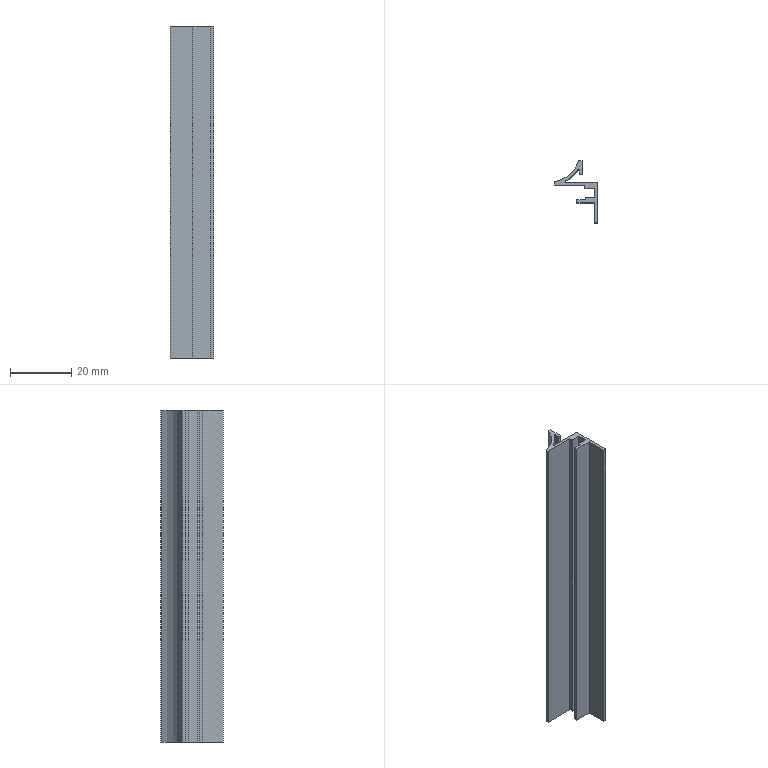Part | SolidWorks | features MoveFace 2, BaseBody 1, ICE 1 | 1 solid | 27 faces | box 14 x 20.3 x 108 mm | volume 5499 mm3 | plane 20 | cylinder 7 | commonest cylinder face diameters 0.387 x2 0.8 x2 0.4 x1 20 x1 22 x1
STEP:
#1=CARTESIAN_POINT('',(-5.304,-0.625,-205.));
#2=VERTEX_POINT('',#1);
#3=CARTESIAN_POINT('',(-5.449,-0.8125,-205.));
#4=VERTEX_POINT('',#3);
#5=CARTESIAN_POINT('',(-5.255,-0.8125,-205.));
#6=DIRECTION('',(0.,0.,1.));
#7=DIRECTION('',(-1.,0.,0.));
#8=AXIS2_PLACEMENT_3D('',#5,#6,#7);
#9=CIRCLE('',#8,0.1937);
#10=EDGE_CURVE('',#2,#4,#9,.T.);
#11=ORIENTED_EDGE('',*,*,#10,.T.);
#12=CARTESIAN_POINT('',(-5.449,-0.8125,-313.));
#13=VERTEX_POINT('',#12);
#14=CARTESIAN_POINT('',(-5.449,-0.8125,230.));
#15=DIRECTION('',(0.,0.,-1.));
#16=VECTOR('',#15,1000.);
#17=LINE('',#14,#16);
#18=EDGE_CURVE('',#4,#13,#17,.T.);
#19=ORIENTED_EDGE('',*,*,#18,.T.);
#20=CARTESIAN_POINT('',(-5.304,-0.625,-313.));
#21=VERTEX_POINT('',#20);
#22=CARTESIAN_POINT('',(-5.255,-0.8125,-313.));
#23=DIRECTION('',(0.,0.,-1.));
#24=DIRECTION('',(1.,0.,0.));
#25=AXIS2_PLACEMENT_3D('',#22,#23,#24);
#26=CIRCLE('',#25,0.1937);
#27=EDGE_CURVE('',#13,#21,#26,.T.);
#28=ORIENTED_EDGE('',*,*,#27,.T.);
#29=CARTESIAN_POINT('',(-5.304,-0.625,230.));
#30=DIRECTION('',(0.,0.,-1.));
#31=VECTOR('',#30,1000.);
#32=LINE('',#29,#31);
#33=EDGE_CURVE('',#2,#21,#32,.T.);
#34=ORIENTED_EDGE('',*,*,#33,.F.);
#35=EDGE_LOOP('',(#11,#19,#28,#34));
#36=FACE_OUTER_BOUND('',#35,.T.);
#37=CARTESIAN_POINT('',(-5.255,-0.8125,230.));
#38=DIRECTION('',(0.,0.,-1.));
#39=DIRECTION('',(-1.,0.,0.));
#40=AXIS2_PLACEMENT_3D('',#37,#38,#39);
#41=CYLINDRICAL_SURFACE('',#40,0.1937);
#42=ADVANCED_FACE('',(#36),#41,.F.);
#43=CARTESIAN_POINT('',(5.,-1.,-313.));
#44=VERTEX_POINT('',#43);
#45=CARTESIAN_POINT('',(5.,-14.3,-313.));
#46=VERTEX_POINT('',#45);
#47=CARTESIAN_POINT('',(5.,29.623,-313.));
#48=DIRECTION('',(0.,-1.,0.));
#49=VECTOR('',#48,1000.);
#50=LINE('',#47,#49);
#51=EDGE_CURVE('',#44,#46,#50,.T.);
#52=ORIENTED_EDGE('',*,*,#51,.F.);
#53=CARTESIAN_POINT('',(5.,-1.,-205.));
#54=VERTEX_POINT('',#53);
#55=CARTESIAN_POINT('',(5.,-1.,230.));
#56=DIRECTION('',(0.,0.,-1.));
#57=VECTOR('',#56,1000.);
#58=LINE('',#55,#57);
#59=EDGE_CURVE('',#54,#44,#58,.T.);
#60=ORIENTED_EDGE('',*,*,#59,.F.);
#61=CARTESIAN_POINT('',(5.,-14.3,-205.));
#62=VERTEX_POINT('',#61);
#63=CARTESIAN_POINT('',(5.,29.623,-205.));
#64=DIRECTION('',(0.,1.,0.));
#65=VECTOR('',#64,1000.);
#66=LINE('',#63,#65);
#67=EDGE_CURVE('',#62,#54,#66,.T.);
#68=ORIENTED_EDGE('',*,*,#67,.F.);
#69=CARTESIAN_POINT('',(5.,-14.3,230.));
#70=DIRECTION('',(0.,0.,1.));
#71=VECTOR('',#70,1000.);
#72=LINE('',#69,#71);
#73=EDGE_CURVE('',#46,#62,#72,.T.);
#74=ORIENTED_EDGE('',*,*,#73,.F.);
#75=EDGE_LOOP('',(#52,#60,#68,#74));
#76=FACE_OUTER_BOUND('',#75,.T.);
#77=CARTESIAN_POINT('',(5.,-14.3,230.));
#78=DIRECTION('',(-1.,0.,0.));
#79=DIRECTION('',(0.,0.,1.));
#80=AXIS2_PLACEMENT_3D('',#77,#78,#79);
#81=PLANE('',#80);
#82=ADVANCED_FACE('',(#76),#81,.F.);
#83=CARTESIAN_POINT('',(-9.,-2.,-313.));
#84=VERTEX_POINT('',#83);
#85=CARTESIAN_POINT('',(-9.,-2.,-205.));
#86=VERTEX_POINT('',#85);
#87=CARTESIAN_POINT('',(-9.,-2.,230.));
#88=DIRECTION('',(0.,0.,1.));
#89=VECTOR('',#88,1000.);
#90=LINE('',#87,#89);
#91=EDGE_CURVE('',#84,#86,#90,.T.);
#92=ORIENTED_EDGE('',*,*,#91,.F.);
#93=CARTESIAN_POINT('',(0.9,-2.,-313.));
#94=VERTEX_POINT('',#93);
#95=CARTESIAN_POINT('',(5.,-2.,-313.));
#96=DIRECTION('',(-1.,0.,0.));
#97=VECTOR('',#96,1000.);
#98=LINE('',#95,#97);
#99=EDGE_CURVE('',#94,#84,#98,.T.);
#100=ORIENTED_EDGE('',*,*,#99,.F.);
#101=CARTESIAN_POINT('',(0.9,-2.,-205.));
#102=VERTEX_POINT('',#101);
#103=CARTESIAN_POINT('',(0.9,-2.,230.));
#104=DIRECTION('',(0.,0.,-1.));
#105=VECTOR('',#104,1000.);
#106=LINE('',#103,#105);
#107=EDGE_CURVE('',#102,#94,#106,.T.);
#108=ORIENTED_EDGE('',*,*,#107,.F.);
#109=CARTESIAN_POINT('',(5.,-2.,-205.));
#110=DIRECTION('',(1.,0.,0.));
#111=VECTOR('',#110,1000.);
#112=LINE('',#109,#111);
#113=EDGE_CURVE('',#86,#102,#112,.T.);
#114=ORIENTED_EDGE('',*,*,#113,.F.);
#115=EDGE_LOOP('',(#92,#100,#108,#114));
#116=FACE_OUTER_BOUND('',#115,.T.);
#117=CARTESIAN_POINT('',(-9.,-2.,230.));
#118=DIRECTION('',(0.,1.,0.));
#119=DIRECTION('',(0.,0.,1.));
#120=AXIS2_PLACEMENT_3D('',#117,#118,#119);
#121=PLANE('',#120);
#122=ADVANCED_FACE('',(#116),#121,.F.);
#123=CARTESIAN_POINT('',(4.,-6.,-205.));
#124=VERTEX_POINT('',#123);
#125=CARTESIAN_POINT('',(4.,-3.,-205.));
#126=VERTEX_POINT('',#125);
#127=CARTESIAN_POINT('',(4.,-3.,-205.));
#128=DIRECTION('',(0.,1.,0.));
#129=VECTOR('',#128,1000.);
#130=LINE('',#127,#129);
#131=EDGE_CURVE('',#124,#126,#130,.T.);
#132=ORIENTED_EDGE('',*,*,#131,.F.);
#133=CARTESIAN_POINT('',(1.,-6.,-205.));
#134=VERTEX_POINT('',#133);
#135=CARTESIAN_POINT('',(4.,-6.,-205.));
#136=DIRECTION('',(1.,0.,0.));
#137=VECTOR('',#136,1000.);
#138=LINE('',#135,#137);
#139=EDGE_CURVE('',#134,#124,#138,.T.);
#140=ORIENTED_EDGE('',*,*,#139,.F.);
#141=CARTESIAN_POINT('',(1.,-6.7,-205.));
#142=VERTEX_POINT('',#141);
#143=CARTESIAN_POINT('',(1.,29.623,-205.));
#144=DIRECTION('',(0.,-1.,0.));
#145=VECTOR('',#144,1000.);
#146=LINE('',#143,#145);
#147=EDGE_CURVE('',#134,#142,#146,.T.);
#148=ORIENTED_EDGE('',*,*,#147,.T.);
#149=CARTESIAN_POINT('',(-1.7,-6.7,-205.));
#150=VERTEX_POINT('',#149);
#151=CARTESIAN_POINT('',(1.,-6.7,-205.));
#152=DIRECTION('',(1.,0.,0.));
#153=VECTOR('',#152,1000.);
#154=LINE('',#151,#153);
#155=EDGE_CURVE('',#150,#142,#154,.T.);
#156=ORIENTED_EDGE('',*,*,#155,.F.);
#157=CARTESIAN_POINT('',(-1.7,-7.7,-205.));
#158=VERTEX_POINT('',#157);
#159=CARTESIAN_POINT('',(-1.7,29.623,-205.));
#160=DIRECTION('',(0.,-1.,0.));
#161=VECTOR('',#160,1000.);
#162=LINE('',#159,#161);
#163=EDGE_CURVE('',#150,#158,#162,.T.);
#164=ORIENTED_EDGE('',*,*,#163,.T.);
#165=CARTESIAN_POINT('',(4.,-7.7,-205.));
#166=VERTEX_POINT('',#165);
#167=CARTESIAN_POINT('',(-1.7,-7.7,-205.));
#168=DIRECTION('',(-1.,0.,0.));
#169=VECTOR('',#168,1000.);
#170=LINE('',#167,#169);
#171=EDGE_CURVE('',#166,#158,#170,.T.);
#172=ORIENTED_EDGE('',*,*,#171,.F.);
#173=CARTESIAN_POINT('',(4.,-14.3,-205.));
#174=VERTEX_POINT('',#173);
#175=CARTESIAN_POINT('',(4.,-7.7,-205.));
#176=DIRECTION('',(0.,1.,0.));
#177=VECTOR('',#176,1000.);
#178=LINE('',#175,#177);
#179=EDGE_CURVE('',#174,#166,#178,.T.);
#180=ORIENTED_EDGE('',*,*,#179,.F.);
#181=CARTESIAN_POINT('',(4.,-14.3,-205.));
#182=DIRECTION('',(-1.,0.,0.));
#183=VECTOR('',#182,1000.);
#184=LINE('',#181,#183);
#185=EDGE_CURVE('',#62,#174,#184,.T.);
#186=ORIENTED_EDGE('',*,*,#185,.F.);
#187=ORIENTED_EDGE('',*,*,#67,.T.);
#188=CARTESIAN_POINT('',(-5.207,-1.,-205.));
#189=VERTEX_POINT('',#188);
#190=CARTESIAN_POINT('',(5.,-1.,-205.));
#191=DIRECTION('',(1.,0.,0.));
#192=VECTOR('',#191,1000.);
#193=LINE('',#190,#192);
#194=EDGE_CURVE('',#189,#54,#193,.T.);
#195=ORIENTED_EDGE('',*,*,#194,.F.);
#196=CARTESIAN_POINT('',(-5.255,-0.8125,-205.));
#197=DIRECTION('',(0.,0.,1.));
#198=DIRECTION('',(-1.,0.,0.));
#199=AXIS2_PLACEMENT_3D('',#196,#197,#198);
#200=CIRCLE('',#199,0.1937);
#201=EDGE_CURVE('',#4,#189,#200,.T.);
#202=ORIENTED_EDGE('',*,*,#201,.F.);
#203=ORIENTED_EDGE('',*,*,#10,.F.);
#204=CARTESIAN_POINT('',(-1.368,3.063,-205.));
#205=VERTEX_POINT('',#204);
#206=CARTESIAN_POINT('',(-10.628,9.,-205.));
#207=DIRECTION('',(0.,0.,1.));
#208=DIRECTION('',(-1.,0.,0.));
#209=AXIS2_PLACEMENT_3D('',#206,#207,#208);
#210=CIRCLE('',#209,11.);
#211=EDGE_CURVE('',#2,#205,#210,.T.);
#212=ORIENTED_EDGE('',*,*,#211,.T.);
#213=CARTESIAN_POINT('',(-1.,2.955,-205.));
#214=VERTEX_POINT('',#213);
#215=CARTESIAN_POINT('',(-1.2,2.955,-205.));
#216=DIRECTION('',(0.,0.,1.));
#217=DIRECTION('',(-1.,0.,0.));
#218=AXIS2_PLACEMENT_3D('',#215,#216,#217);
#219=CIRCLE('',#218,0.2);
#220=EDGE_CURVE('',#214,#205,#219,.T.);
#221=ORIENTED_EDGE('',*,*,#220,.F.);
#222=CARTESIAN_POINT('',(-1.,1.5,-205.));
#223=VERTEX_POINT('',#222);
#224=CARTESIAN_POINT('',(-1.,2.955,-205.));
#225=DIRECTION('',(0.,1.,0.));
#226=VECTOR('',#225,1000.);
#227=LINE('',#224,#226);
#228=EDGE_CURVE('',#223,#214,#227,.T.);
#229=ORIENTED_EDGE('',*,*,#228,.F.);
#230=CARTESIAN_POINT('',(0.,1.5,-205.));
#231=VERTEX_POINT('',#230);
#232=CARTESIAN_POINT('',(-1.,1.5,-205.));
#233=DIRECTION('',(-1.,0.,0.));
#234=VECTOR('',#233,1000.);
#235=LINE('',#232,#234);
#236=EDGE_CURVE('',#231,#223,#235,.T.);
#237=ORIENTED_EDGE('',*,*,#236,.F.);
#238=CARTESIAN_POINT('',(0.,6.,-205.));
#239=VERTEX_POINT('',#238);
#240=CARTESIAN_POINT('',(0.,1.5,-205.));
#241=DIRECTION('',(0.,-1.,0.));
#242=VECTOR('',#241,1000.);
#243=LINE('',#240,#242);
#244=EDGE_CURVE('',#239,#231,#243,.T.);
#245=ORIENTED_EDGE('',*,*,#244,.F.);
#246=CARTESIAN_POINT('',(-0.8,6.,-205.));
#247=VERTEX_POINT('',#246);
#248=CARTESIAN_POINT('',(0.,6.,-205.));
#249=DIRECTION('',(1.,0.,0.));
#250=VECTOR('',#249,1000.);
#251=LINE('',#248,#250);
#252=EDGE_CURVE('',#247,#239,#251,.T.);
#253=ORIENTED_EDGE('',*,*,#252,.F.);
#254=CARTESIAN_POINT('',(-1.178,5.731,-205.));
#255=VERTEX_POINT('',#254);
#256=CARTESIAN_POINT('',(-0.8,5.6,-205.));
#257=DIRECTION('',(0.,0.,1.));
#258=DIRECTION('',(-1.,0.,0.));
#259=AXIS2_PLACEMENT_3D('',#256,#257,#258);
#260=CIRCLE('',#259,0.4);
#261=EDGE_CURVE('',#247,#255,#260,.T.);
#262=ORIENTED_EDGE('',*,*,#261,.T.);
#263=CARTESIAN_POINT('',(-8.678,-0.8077,-205.));
#264=VERTEX_POINT('',#263);
#265=CARTESIAN_POINT('',(-10.628,9.,-205.));
#266=DIRECTION('',(0.,0.,1.));
#267=DIRECTION('',(-1.,0.,0.));
#268=AXIS2_PLACEMENT_3D('',#265,#266,#267);
#269=CIRCLE('',#268,10.);
#270=EDGE_CURVE('',#264,#255,#269,.T.);
#271=ORIENTED_EDGE('',*,*,#270,.F.);
#272=CARTESIAN_POINT('',(-9.,-1.2,-205.));
#273=VERTEX_POINT('',#272);
#274=CARTESIAN_POINT('',(-8.6,-1.2,-205.));
#275=DIRECTION('',(0.,0.,1.));
#276=DIRECTION('',(-1.,0.,0.));
#277=AXIS2_PLACEMENT_3D('',#274,#275,#276);
#278=CIRCLE('',#277,0.4);
#279=EDGE_CURVE('',#264,#273,#278,.T.);
#280=ORIENTED_EDGE('',*,*,#279,.T.);
#281=CARTESIAN_POINT('',(-9.,29.623,-205.));
#282=DIRECTION('',(0.,-1.,0.));
#283=VECTOR('',#282,1000.);
#284=LINE('',#281,#283);
#285=EDGE_CURVE('',#273,#86,#284,.T.);
#286=ORIENTED_EDGE('',*,*,#285,.T.);
#287=ORIENTED_EDGE('',*,*,#113,.T.);
#288=CARTESIAN_POINT('',(0.9,-3.,-205.));
#289=VERTEX_POINT('',#288);
#290=CARTESIAN_POINT('',(0.9,-2.,-205.));
#291=DIRECTION('',(0.,1.,0.));
#292=VECTOR('',#291,1000.);
#293=LINE('',#290,#292);
#294=EDGE_CURVE('',#289,#102,#293,.T.);
#295=ORIENTED_EDGE('',*,*,#294,.F.);
#296=CARTESIAN_POINT('',(0.9,-3.,-205.));
#297=DIRECTION('',(-1.,0.,0.));
#298=VECTOR('',#297,1000.);
#299=LINE('',#296,#298);
#300=EDGE_CURVE('',#126,#289,#299,.T.);
#301=ORIENTED_EDGE('',*,*,#300,.F.);
#302=EDGE_LOOP('',(#132,#140,#148,#156,#164,#172,#180,#186,#187,#195,#202,#203,#212,#221,#229,#237,#245,#253,#262,#271,#280,#286,#287,#295,#301));
#303=FACE_OUTER_BOUND('',#302,.T.);
#304=CARTESIAN_POINT('',(5.,29.623,-205.));
#305=DIRECTION('',(0.,0.,-1.));
#306=DIRECTION('',(-1.,0.,0.));
#307=AXIS2_PLACEMENT_3D('',#304,#305,#306);
#308=PLANE('',#307);
#309=ADVANCED_FACE('',(#303),#308,.F.);
#310=ORIENTED_EDGE('',*,*,#185,.T.);
#311=CARTESIAN_POINT('',(4.,-14.3,-313.));
#312=VERTEX_POINT('',#311);
#313=CARTESIAN_POINT('',(4.,-14.3,230.));
#314=DIRECTION('',(0.,0.,1.));
#315=VECTOR('',#314,1000.);
#316=LINE('',#313,#315);
#317=EDGE_CURVE('',#312,#174,#316,.T.);
#318=ORIENTED_EDGE('',*,*,#317,.F.);
#319=CARTESIAN_POINT('',(5.,-14.3,-313.));
#320=DIRECTION('',(-1.,0.,0.));
#321=VECTOR('',#320,1000.);
#322=LINE('',#319,#321);
#323=EDGE_CURVE('',#46,#312,#322,.T.);
#324=ORIENTED_EDGE('',*,*,#323,.F.);
#325=ORIENTED_EDGE('',*,*,#73,.T.);
#326=EDGE_LOOP('',(#310,#318,#324,#325));
#327=FACE_OUTER_BOUND('',#326,.T.);
#328=CARTESIAN_POINT('',(4.,-14.3,230.));
#329=DIRECTION('',(0.,1.,0.));
#330=DIRECTION('',(0.,0.,1.));
#331=AXIS2_PLACEMENT_3D('',#328,#329,#330);
#332=PLANE('',#331);
#333=ADVANCED_FACE('',(#327),#332,.F.);
#334=ORIENTED_EDGE('',*,*,#51,.T.);
#335=ORIENTED_EDGE('',*,*,#323,.T.);
#336=CARTESIAN_POINT('',(4.,-7.7,-313.));
#337=VERTEX_POINT('',#336);
#338=CARTESIAN_POINT('',(4.,-7.7,-313.));
#339=DIRECTION('',(0.,-1.,0.));
#340=VECTOR('',#339,1000.);
#341=LINE('',#338,#340);
#342=EDGE_CURVE('',#337,#312,#341,.T.);
#343=ORIENTED_EDGE('',*,*,#342,.F.);
#344=CARTESIAN_POINT('',(-1.7,-7.7,-313.));
#345=VERTEX_POINT('',#344);
#346=CARTESIAN_POINT('',(-1.7,-7.7,-313.));
#347=DIRECTION('',(1.,0.,0.));
#348=VECTOR('',#347,1000.);
#349=LINE('',#346,#348);
#350=EDGE_CURVE('',#345,#337,#349,.T.);
#351=ORIENTED_EDGE('',*,*,#350,.F.);
#352=CARTESIAN_POINT('',(-1.7,-6.7,-313.));
#353=VERTEX_POINT('',#352);
#354=CARTESIAN_POINT('',(-1.7,29.623,-313.));
#355=DIRECTION('',(0.,1.,0.));
#356=VECTOR('',#355,1000.);
#357=LINE('',#354,#356);
#358=EDGE_CURVE('',#345,#353,#357,.T.);
#359=ORIENTED_EDGE('',*,*,#358,.T.);
#360=CARTESIAN_POINT('',(1.,-6.7,-313.));
#361=VERTEX_POINT('',#360);
#362=CARTESIAN_POINT('',(1.,-6.7,-313.));
#363=DIRECTION('',(-1.,0.,0.));
#364=VECTOR('',#363,1000.);
#365=LINE('',#362,#364);
#366=EDGE_CURVE('',#361,#353,#365,.T.);
#367=ORIENTED_EDGE('',*,*,#366,.F.);
#368=CARTESIAN_POINT('',(1.,-6.,-313.));
#369=VERTEX_POINT('',#368);
#370=CARTESIAN_POINT('',(1.,29.623,-313.));
#371=DIRECTION('',(0.,1.,0.));
#372=VECTOR('',#371,1000.);
#373=LINE('',#370,#372);
#374=EDGE_CURVE('',#361,#369,#373,.T.);
#375=ORIENTED_EDGE('',*,*,#374,.T.);
#376=CARTESIAN_POINT('',(4.,-6.,-313.));
#377=VERTEX_POINT('',#376);
#378=CARTESIAN_POINT('',(4.,-6.,-313.));
#379=DIRECTION('',(-1.,0.,0.));
#380=VECTOR('',#379,1000.);
#381=LINE('',#378,#380);
#382=EDGE_CURVE('',#377,#369,#381,.T.);
#383=ORIENTED_EDGE('',*,*,#382,.F.);
#384=CARTESIAN_POINT('',(4.,-3.,-313.));
#385=VERTEX_POINT('',#384);
#386=CARTESIAN_POINT('',(4.,-3.,-313.));
#387=DIRECTION('',(0.,-1.,0.));
#388=VECTOR('',#387,1000.);
#389=LINE('',#386,#388);
#390=EDGE_CURVE('',#385,#377,#389,.T.);
#391=ORIENTED_EDGE('',*,*,#390,.F.);
#392=CARTESIAN_POINT('',(0.9,-3.,-313.));
#393=VERTEX_POINT('',#392);
#394=CARTESIAN_POINT('',(0.9,-3.,-313.));
#395=DIRECTION('',(1.,0.,0.));
#396=VECTOR('',#395,1000.);
#397=LINE('',#394,#396);
#398=EDGE_CURVE('',#393,#385,#397,.T.);
#399=ORIENTED_EDGE('',*,*,#398,.F.);
#400=CARTESIAN_POINT('',(0.9,-2.,-313.));
#401=DIRECTION('',(0.,-1.,0.));
#402=VECTOR('',#401,1000.);
#403=LINE('',#400,#402);
#404=EDGE_CURVE('',#94,#393,#403,.T.);
#405=ORIENTED_EDGE('',*,*,#404,.F.);
#406=ORIENTED_EDGE('',*,*,#99,.T.);
#407=CARTESIAN_POINT('',(-9.,-1.2,-313.));
#408=VERTEX_POINT('',#407);
#409=CARTESIAN_POINT('',(-9.,-1.2,-313.));
#410=DIRECTION('',(0.,-1.,0.));
#411=VECTOR('',#410,1000.);
#412=LINE('',#409,#411);
#413=EDGE_CURVE('',#408,#84,#412,.T.);
#414=ORIENTED_EDGE('',*,*,#413,.F.);
#415=CARTESIAN_POINT('',(-8.678,-0.8077,-313.));
#416=VERTEX_POINT('',#415);
#417=CARTESIAN_POINT('',(-8.6,-1.2,-313.));
#418=DIRECTION('',(0.,0.,-1.));
#419=DIRECTION('',(1.,0.,0.));
#420=AXIS2_PLACEMENT_3D('',#417,#418,#419);
#421=CIRCLE('',#420,0.4);
#422=EDGE_CURVE('',#408,#416,#421,.T.);
#423=ORIENTED_EDGE('',*,*,#422,.T.);
#424=CARTESIAN_POINT('',(-1.178,5.731,-313.));
#425=VERTEX_POINT('',#424);
#426=CARTESIAN_POINT('',(-10.628,9.,-313.));
#427=DIRECTION('',(0.,0.,-1.));
#428=DIRECTION('',(1.,0.,0.));
#429=AXIS2_PLACEMENT_3D('',#426,#427,#428);
#430=CIRCLE('',#429,10.);
#431=EDGE_CURVE('',#425,#416,#430,.T.);
#432=ORIENTED_EDGE('',*,*,#431,.F.);
#433=CARTESIAN_POINT('',(-0.8,6.,-313.));
#434=VERTEX_POINT('',#433);
#435=CARTESIAN_POINT('',(-0.8,5.6,-313.));
#436=DIRECTION('',(0.,0.,-1.));
#437=DIRECTION('',(1.,0.,0.));
#438=AXIS2_PLACEMENT_3D('',#435,#436,#437);
#439=CIRCLE('',#438,0.4);
#440=EDGE_CURVE('',#425,#434,#439,.T.);
#441=ORIENTED_EDGE('',*,*,#440,.T.);
#442=CARTESIAN_POINT('',(0.,6.,-313.));
#443=VERTEX_POINT('',#442);
#444=CARTESIAN_POINT('',(0.,6.,-313.));
#445=DIRECTION('',(-1.,0.,0.));
#446=VECTOR('',#445,1000.);
#447=LINE('',#444,#446);
#448=EDGE_CURVE('',#443,#434,#447,.T.);
#449=ORIENTED_EDGE('',*,*,#448,.F.);
#450=CARTESIAN_POINT('',(0.,1.5,-313.));
#451=VERTEX_POINT('',#450);
#452=CARTESIAN_POINT('',(0.,1.5,-313.));
#453=DIRECTION('',(0.,1.,0.));
#454=VECTOR('',#453,1000.);
#455=LINE('',#452,#454);
#456=EDGE_CURVE('',#451,#443,#455,.T.);
#457=ORIENTED_EDGE('',*,*,#456,.F.);
#458=CARTESIAN_POINT('',(-1.,1.5,-313.));
#459=VERTEX_POINT('',#458);
#460=CARTESIAN_POINT('',(-1.,1.5,-313.));
#461=DIRECTION('',(1.,0.,0.));
#462=VECTOR('',#461,1000.);
#463=LINE('',#460,#462);
#464=EDGE_CURVE('',#459,#451,#463,.T.);
#465=ORIENTED_EDGE('',*,*,#464,.F.);
#466=CARTESIAN_POINT('',(-1.,2.955,-313.));
#467=VERTEX_POINT('',#466);
#468=CARTESIAN_POINT('',(-1.,2.955,-313.));
#469=DIRECTION('',(0.,-1.,0.));
#470=VECTOR('',#469,1000.);
#471=LINE('',#468,#470);
#472=EDGE_CURVE('',#467,#459,#471,.T.);
#473=ORIENTED_EDGE('',*,*,#472,.F.);
#474=CARTESIAN_POINT('',(-1.368,3.063,-313.));
#475=VERTEX_POINT('',#474);
#476=CARTESIAN_POINT('',(-1.2,2.955,-313.));
#477=DIRECTION('',(0.,0.,-1.));
#478=DIRECTION('',(1.,0.,0.));
#479=AXIS2_PLACEMENT_3D('',#476,#477,#478);
#480=CIRCLE('',#479,0.2);
#481=EDGE_CURVE('',#475,#467,#480,.T.);
#482=ORIENTED_EDGE('',*,*,#481,.F.);
#483=CARTESIAN_POINT('',(-10.628,9.,-313.));
#484=DIRECTION('',(0.,0.,-1.));
#485=DIRECTION('',(1.,0.,0.));
#486=AXIS2_PLACEMENT_3D('',#483,#484,#485);
#487=CIRCLE('',#486,11.);
#488=EDGE_CURVE('',#475,#21,#487,.T.);
#489=ORIENTED_EDGE('',*,*,#488,.T.);
#490=ORIENTED_EDGE('',*,*,#27,.F.);
#491=CARTESIAN_POINT('',(-5.207,-1.,-313.));
#492=VERTEX_POINT('',#491);
#493=CARTESIAN_POINT('',(-5.255,-0.8125,-313.));
#494=DIRECTION('',(0.,0.,-1.));
#495=DIRECTION('',(1.,0.,0.));
#496=AXIS2_PLACEMENT_3D('',#493,#494,#495);
#497=CIRCLE('',#496,0.1937);
#498=EDGE_CURVE('',#492,#13,#497,.T.);
#499=ORIENTED_EDGE('',*,*,#498,.F.);
#500=CARTESIAN_POINT('',(5.,-1.,-313.));
#501=DIRECTION('',(-1.,0.,0.));
#502=VECTOR('',#501,1000.);
#503=LINE('',#500,#502);
#504=EDGE_CURVE('',#44,#492,#503,.T.);
#505=ORIENTED_EDGE('',*,*,#504,.F.);
#506=EDGE_LOOP('',(#334,#335,#343,#351,#359,#367,#375,#383,#391,#399,#405,#406,#414,#423,#432,#441,#449,#457,#465,#473,#482,#489,#490,#499,#505));
#507=FACE_OUTER_BOUND('',#506,.T.);
#508=CARTESIAN_POINT('',(5.,29.623,-313.));
#509=DIRECTION('',(0.,0.,1.));
#510=DIRECTION('',(1.,0.,0.));
#511=AXIS2_PLACEMENT_3D('',#508,#509,#510);
#512=PLANE('',#511);
#513=ADVANCED_FACE('',(#507),#512,.F.);
#514=ORIENTED_EDGE('',*,*,#59,.T.);
#515=ORIENTED_EDGE('',*,*,#504,.T.);
#516=CARTESIAN_POINT('',(-5.207,-1.,230.));
#517=DIRECTION('',(0.,0.,-1.));
#518=VECTOR('',#517,1000.);
#519=LINE('',#516,#518);
#520=EDGE_CURVE('',#189,#492,#519,.T.);
#521=ORIENTED_EDGE('',*,*,#520,.F.);
#522=ORIENTED_EDGE('',*,*,#194,.T.);
#523=EDGE_LOOP('',(#514,#515,#521,#522));
#524=FACE_OUTER_BOUND('',#523,.T.);
#525=CARTESIAN_POINT('',(5.,-1.,230.));
#526=DIRECTION('',(0.,-1.,0.));
#527=DIRECTION('',(0.,0.,-1.));
#528=AXIS2_PLACEMENT_3D('',#525,#526,#527);
#529=PLANE('',#528);
#530=ADVANCED_FACE('',(#524),#529,.F.);
#531=CARTESIAN_POINT('',(-9.,-1.2,230.));
#532=DIRECTION('',(0.,0.,1.));
#533=VECTOR('',#532,1000.);
#534=LINE('',#531,#533);
#535=EDGE_CURVE('',#408,#273,#534,.T.);
#536=ORIENTED_EDGE('',*,*,#535,.F.);
#537=ORIENTED_EDGE('',*,*,#413,.T.);
#538=ORIENTED_EDGE('',*,*,#91,.T.);
#539=ORIENTED_EDGE('',*,*,#285,.F.);
#540=EDGE_LOOP('',(#536,#537,#538,#539));
#541=FACE_OUTER_BOUND('',#540,.T.);
#542=CARTESIAN_POINT('',(-9.,-1.2,230.));
#543=DIRECTION('',(1.,0.,0.));
#544=DIRECTION('',(0.,0.,-1.));
#545=AXIS2_PLACEMENT_3D('',#542,#543,#544);
#546=PLANE('',#545);
#547=ADVANCED_FACE('',(#541),#546,.F.);
#548=ORIENTED_EDGE('',*,*,#294,.T.);
#549=ORIENTED_EDGE('',*,*,#107,.T.);
#550=ORIENTED_EDGE('',*,*,#404,.T.);
#551=CARTESIAN_POINT('',(0.9,-3.,230.));
#552=DIRECTION('',(0.,0.,-1.));
#553=VECTOR('',#552,1000.);
#554=LINE('',#551,#553);
#555=EDGE_CURVE('',#289,#393,#554,.T.);
#556=ORIENTED_EDGE('',*,*,#555,.F.);
#557=EDGE_LOOP('',(#548,#549,#550,#556));
#558=FACE_OUTER_BOUND('',#557,.T.);
#559=CARTESIAN_POINT('',(0.9,-2.,230.));
#560=DIRECTION('',(1.,0.,0.));
#561=DIRECTION('',(0.,0.,-1.));
#562=AXIS2_PLACEMENT_3D('',#559,#560,#561);
#563=PLANE('',#562);
#564=ADVANCED_FACE('',(#558),#563,.F.);
#565=ORIENTED_EDGE('',*,*,#300,.T.);
#566=ORIENTED_EDGE('',*,*,#555,.T.);
#567=ORIENTED_EDGE('',*,*,#398,.T.);
#568=CARTESIAN_POINT('',(4.,-3.,230.));
#569=DIRECTION('',(0.,0.,-1.));
#570=VECTOR('',#569,1000.);
#571=LINE('',#568,#570);
#572=EDGE_CURVE('',#126,#385,#571,.T.);
#573=ORIENTED_EDGE('',*,*,#572,.F.);
#574=EDGE_LOOP('',(#565,#566,#567,#573));
#575=FACE_OUTER_BOUND('',#574,.T.);
#576=CARTESIAN_POINT('',(0.9,-3.,230.));
#577=DIRECTION('',(0.,1.,0.));
#578=DIRECTION('',(0.,0.,1.));
#579=AXIS2_PLACEMENT_3D('',#576,#577,#578);
#580=PLANE('',#579);
#581=ADVANCED_FACE('',(#575),#580,.F.);
#582=ORIENTED_EDGE('',*,*,#131,.T.);
#583=ORIENTED_EDGE('',*,*,#572,.T.);
#584=ORIENTED_EDGE('',*,*,#390,.T.);
#585=CARTESIAN_POINT('',(4.,-6.,230.));
#586=DIRECTION('',(0.,0.,-1.));
#587=VECTOR('',#586,1000.);
#588=LINE('',#585,#587);
#589=EDGE_CURVE('',#124,#377,#588,.T.);
#590=ORIENTED_EDGE('',*,*,#589,.F.);
#591=EDGE_LOOP('',(#582,#583,#584,#590));
#592=FACE_OUTER_BOUND('',#591,.T.);
#593=CARTESIAN_POINT('',(4.,-3.,230.));
#594=DIRECTION('',(1.,0.,0.));
#595=DIRECTION('',(0.,0.,-1.));
#596=AXIS2_PLACEMENT_3D('',#593,#594,#595);
#597=PLANE('',#596);
#598=ADVANCED_FACE('',(#592),#597,.F.);
#599=ORIENTED_EDGE('',*,*,#139,.T.);
#600=ORIENTED_EDGE('',*,*,#589,.T.);
#601=ORIENTED_EDGE('',*,*,#382,.T.);
#602=CARTESIAN_POINT('',(1.,-6.,230.));
#603=DIRECTION('',(0.,0.,-1.));
#604=VECTOR('',#603,1000.);
#605=LINE('',#602,#604);
#606=EDGE_CURVE('',#134,#369,#605,.T.);
#607=ORIENTED_EDGE('',*,*,#606,.F.);
#608=EDGE_LOOP('',(#599,#600,#601,#607));
#609=FACE_OUTER_BOUND('',#608,.T.);
#610=CARTESIAN_POINT('',(4.,-6.,230.));
#611=DIRECTION('',(0.,-1.,0.));
#612=DIRECTION('',(0.,0.,-1.));
#613=AXIS2_PLACEMENT_3D('',#610,#611,#612);
#614=PLANE('',#613);
#615=ADVANCED_FACE('',(#609),#614,.F.);
#616=ORIENTED_EDGE('',*,*,#155,.T.);
#617=CARTESIAN_POINT('',(1.,-6.7,230.));
#618=DIRECTION('',(0.,0.,1.));
#619=VECTOR('',#618,1000.);
#620=LINE('',#617,#619);
#621=EDGE_CURVE('',#361,#142,#620,.T.);
#622=ORIENTED_EDGE('',*,*,#621,.F.);
#623=ORIENTED_EDGE('',*,*,#366,.T.);
#624=CARTESIAN_POINT('',(-1.7,-6.7,230.));
#625=DIRECTION('',(0.,0.,-1.));
#626=VECTOR('',#625,1000.);
#627=LINE('',#624,#626);
#628=EDGE_CURVE('',#150,#353,#627,.T.);
#629=ORIENTED_EDGE('',*,*,#628,.F.);
#630=EDGE_LOOP('',(#616,#622,#623,#629));
#631=FACE_OUTER_BOUND('',#630,.T.);
#632=CARTESIAN_POINT('',(1.,-6.7,230.));
#633=DIRECTION('',(0.,-1.,0.));
#634=DIRECTION('',(0.,0.,-1.));
#635=AXIS2_PLACEMENT_3D('',#632,#633,#634);
#636=PLANE('',#635);
#637=ADVANCED_FACE('',(#631),#636,.F.);
#638=ORIENTED_EDGE('',*,*,#171,.T.);
#639=CARTESIAN_POINT('',(-1.7,-7.7,230.));
#640=DIRECTION('',(0.,0.,1.));
#641=VECTOR('',#640,1000.);
#642=LINE('',#639,#641);
#643=EDGE_CURVE('',#345,#158,#642,.T.);
#644=ORIENTED_EDGE('',*,*,#643,.F.);
#645=ORIENTED_EDGE('',*,*,#350,.T.);
#646=CARTESIAN_POINT('',(4.,-7.7,230.));
#647=DIRECTION('',(0.,0.,-1.));
#648=VECTOR('',#647,1000.);
#649=LINE('',#646,#648);
#650=EDGE_CURVE('',#166,#337,#649,.T.);
#651=ORIENTED_EDGE('',*,*,#650,.F.);
#652=EDGE_LOOP('',(#638,#644,#645,#651));
#653=FACE_OUTER_BOUND('',#652,.T.);
#654=CARTESIAN_POINT('',(-1.7,-7.7,230.));
#655=DIRECTION('',(0.,1.,0.));
#656=DIRECTION('',(0.,0.,1.));
#657=AXIS2_PLACEMENT_3D('',#654,#655,#656);
#658=PLANE('',#657);
#659=ADVANCED_FACE('',(#653),#658,.F.);
#660=ORIENTED_EDGE('',*,*,#179,.T.);
#661=ORIENTED_EDGE('',*,*,#650,.T.);
#662=ORIENTED_EDGE('',*,*,#342,.T.);
#663=ORIENTED_EDGE('',*,*,#317,.T.);
#664=EDGE_LOOP('',(#660,#661,#662,#663));
#665=FACE_OUTER_BOUND('',#664,.T.);
#666=CARTESIAN_POINT('',(4.,-7.7,230.));
#667=DIRECTION('',(1.,0.,0.));
#668=DIRECTION('',(0.,0.,-1.));
#669=AXIS2_PLACEMENT_3D('',#666,#667,#668);
#670=PLANE('',#669);
#671=ADVANCED_FACE('',(#665),#670,.F.);
#672=ORIENTED_EDGE('',*,*,#18,.F.);
#673=ORIENTED_EDGE('',*,*,#201,.T.);
#674=ORIENTED_EDGE('',*,*,#520,.T.);
#675=ORIENTED_EDGE('',*,*,#498,.T.);
#676=EDGE_LOOP('',(#672,#673,#674,#675));
#677=FACE_OUTER_BOUND('',#676,.T.);
#678=CARTESIAN_POINT('',(-5.255,-0.8125,230.));
#679=DIRECTION('',(0.,0.,-1.));
#680=DIRECTION('',(-1.,0.,0.));
#681=AXIS2_PLACEMENT_3D('',#678,#679,#680);
#682=CYLINDRICAL_SURFACE('',#681,0.1937);
#683=ADVANCED_FACE('',(#677),#682,.F.);
#684=CARTESIAN_POINT('',(-1.,2.955,230.));
#685=DIRECTION('',(0.,0.,1.));
#686=VECTOR('',#685,1000.);
#687=LINE('',#684,#686);
#688=EDGE_CURVE('',#467,#214,#687,.T.);
#689=ORIENTED_EDGE('',*,*,#688,.F.);
#690=ORIENTED_EDGE('',*,*,#472,.T.);
#691=CARTESIAN_POINT('',(-1.,1.5,230.));
#692=DIRECTION('',(0.,0.,-1.));
#693=VECTOR('',#692,1000.);
#694=LINE('',#691,#693);
#695=EDGE_CURVE('',#223,#459,#694,.T.);
#696=ORIENTED_EDGE('',*,*,#695,.F.);
#697=ORIENTED_EDGE('',*,*,#228,.T.);
#698=EDGE_LOOP('',(#689,#690,#696,#697));
#699=FACE_OUTER_BOUND('',#698,.T.);
#700=CARTESIAN_POINT('',(-1.,2.955,230.));
#701=DIRECTION('',(1.,0.,0.));
#702=DIRECTION('',(0.,0.,-1.));
#703=AXIS2_PLACEMENT_3D('',#700,#701,#702);
#704=PLANE('',#703);
#705=ADVANCED_FACE('',(#699),#704,.F.);
#706=ORIENTED_EDGE('',*,*,#488,.F.);
#707=CARTESIAN_POINT('',(-1.368,3.063,230.));
#708=DIRECTION('',(0.,0.,1.));
#709=VECTOR('',#708,1000.);
#710=LINE('',#707,#709);
#711=EDGE_CURVE('',#475,#205,#710,.T.);
#712=ORIENTED_EDGE('',*,*,#711,.T.);
#713=ORIENTED_EDGE('',*,*,#211,.F.);
#714=ORIENTED_EDGE('',*,*,#33,.T.);
#715=EDGE_LOOP('',(#706,#712,#713,#714));
#716=FACE_OUTER_BOUND('',#715,.T.);
#717=CARTESIAN_POINT('',(-10.628,9.,230.));
#718=DIRECTION('',(0.,0.,-1.));
#719=DIRECTION('',(-1.,0.,0.));
#720=AXIS2_PLACEMENT_3D('',#717,#718,#719);
#721=CYLINDRICAL_SURFACE('',#720,11.);
#722=ADVANCED_FACE('',(#716),#721,.T.);
#723=CARTESIAN_POINT('',(-1.178,5.731,230.));
#724=DIRECTION('',(0.,0.,1.));
#725=VECTOR('',#724,1000.);
#726=LINE('',#723,#725);
#727=EDGE_CURVE('',#425,#255,#726,.T.);
#728=ORIENTED_EDGE('',*,*,#727,.F.);
#729=ORIENTED_EDGE('',*,*,#431,.T.);
#730=CARTESIAN_POINT('',(-8.678,-0.8077,230.));
#731=DIRECTION('',(0.,0.,-1.));
#732=VECTOR('',#731,1000.);
#733=LINE('',#730,#732);
#734=EDGE_CURVE('',#264,#416,#733,.T.);
#735=ORIENTED_EDGE('',*,*,#734,.F.);
#736=ORIENTED_EDGE('',*,*,#270,.T.);
#737=EDGE_LOOP('',(#728,#729,#735,#736));
#738=FACE_OUTER_BOUND('',#737,.T.);
#739=CARTESIAN_POINT('',(-10.628,9.,230.));
#740=DIRECTION('',(0.,0.,-1.));
#741=DIRECTION('',(-1.,0.,0.));
#742=AXIS2_PLACEMENT_3D('',#739,#740,#741);
#743=CYLINDRICAL_SURFACE('',#742,10.);
#744=ADVANCED_FACE('',(#738),#743,.F.);
#745=CARTESIAN_POINT('',(0.,1.5,230.));
#746=DIRECTION('',(0.,0.,1.));
#747=VECTOR('',#746,1000.);
#748=LINE('',#745,#747);
#749=EDGE_CURVE('',#451,#231,#748,.T.);
#750=ORIENTED_EDGE('',*,*,#749,.F.);
#751=ORIENTED_EDGE('',*,*,#456,.T.);
#752=CARTESIAN_POINT('',(0.,6.,230.));
#753=DIRECTION('',(0.,0.,-1.));
#754=VECTOR('',#753,1000.);
#755=LINE('',#752,#754);
#756=EDGE_CURVE('',#239,#443,#755,.T.);
#757=ORIENTED_EDGE('',*,*,#756,.F.);
#758=ORIENTED_EDGE('',*,*,#244,.T.);
#759=EDGE_LOOP('',(#750,#751,#757,#758));
#760=FACE_OUTER_BOUND('',#759,.T.);
#761=CARTESIAN_POINT('',(0.,1.5,230.));
#762=DIRECTION('',(-1.,0.,0.));
#763=DIRECTION('',(0.,0.,1.));
#764=AXIS2_PLACEMENT_3D('',#761,#762,#763);
#765=PLANE('',#764);
#766=ADVANCED_FACE('',(#760),#765,.F.);
#767=ORIENTED_EDGE('',*,*,#422,.F.);
#768=ORIENTED_EDGE('',*,*,#535,.T.);
#769=ORIENTED_EDGE('',*,*,#279,.F.);
#770=ORIENTED_EDGE('',*,*,#734,.T.);
#771=EDGE_LOOP('',(#767,#768,#769,#770));
#772=FACE_OUTER_BOUND('',#771,.T.);
#773=CARTESIAN_POINT('',(-8.6,-1.2,230.));
#774=DIRECTION('',(0.,0.,-1.));
#775=DIRECTION('',(-1.,0.,0.));
#776=AXIS2_PLACEMENT_3D('',#773,#774,#775);
#777=CYLINDRICAL_SURFACE('',#776,0.4);
#778=ADVANCED_FACE('',(#772),#777,.T.);
#779=ORIENTED_EDGE('',*,*,#147,.F.);
#780=ORIENTED_EDGE('',*,*,#606,.T.);
#781=ORIENTED_EDGE('',*,*,#374,.F.);
#782=ORIENTED_EDGE('',*,*,#621,.T.);
#783=EDGE_LOOP('',(#779,#780,#781,#782));
#784=FACE_OUTER_BOUND('',#783,.T.);
#785=CARTESIAN_POINT('',(1.,-6.,230.));
#786=DIRECTION('',(1.,0.,0.));
#787=DIRECTION('',(0.,0.,-1.));
#788=AXIS2_PLACEMENT_3D('',#785,#786,#787);
#789=PLANE('',#788);
#790=ADVANCED_FACE('',(#784),#789,.F.);
#791=ORIENTED_EDGE('',*,*,#163,.F.);
#792=ORIENTED_EDGE('',*,*,#628,.T.);
#793=ORIENTED_EDGE('',*,*,#358,.F.);
#794=ORIENTED_EDGE('',*,*,#643,.T.);
#795=EDGE_LOOP('',(#791,#792,#793,#794));
#796=FACE_OUTER_BOUND('',#795,.T.);
#797=CARTESIAN_POINT('',(-1.7,-6.7,230.));
#798=DIRECTION('',(1.,0.,0.));
#799=DIRECTION('',(0.,0.,-1.));
#800=AXIS2_PLACEMENT_3D('',#797,#798,#799);
#801=PLANE('',#800);
#802=ADVANCED_FACE('',(#796),#801,.F.);
#803=ORIENTED_EDGE('',*,*,#711,.F.);
#804=ORIENTED_EDGE('',*,*,#481,.T.);
#805=ORIENTED_EDGE('',*,*,#688,.T.);
#806=ORIENTED_EDGE('',*,*,#220,.T.);
#807=EDGE_LOOP('',(#803,#804,#805,#806));
#808=FACE_OUTER_BOUND('',#807,.T.);
#809=CARTESIAN_POINT('',(-1.2,2.955,230.));
#810=DIRECTION('',(0.,0.,-1.));
#811=DIRECTION('',(-1.,0.,0.));
#812=AXIS2_PLACEMENT_3D('',#809,#810,#811);
#813=CYLINDRICAL_SURFACE('',#812,0.2);
#814=ADVANCED_FACE('',(#808),#813,.F.);
#815=ORIENTED_EDGE('',*,*,#695,.T.);
#816=ORIENTED_EDGE('',*,*,#464,.T.);
#817=ORIENTED_EDGE('',*,*,#749,.T.);
#818=ORIENTED_EDGE('',*,*,#236,.T.);
#819=EDGE_LOOP('',(#815,#816,#817,#818));
#820=FACE_OUTER_BOUND('',#819,.T.);
#821=CARTESIAN_POINT('',(-1.,1.5,230.));
#822=DIRECTION('',(0.,1.,0.));
#823=DIRECTION('',(0.,0.,1.));
#824=AXIS2_PLACEMENT_3D('',#821,#822,#823);
#825=PLANE('',#824);
#826=ADVANCED_FACE('',(#820),#825,.F.);
#827=ORIENTED_EDGE('',*,*,#440,.F.);
#828=ORIENTED_EDGE('',*,*,#727,.T.);
#829=ORIENTED_EDGE('',*,*,#261,.F.);
#830=CARTESIAN_POINT('',(-0.8,6.,230.));
#831=DIRECTION('',(0.,0.,-1.));
#832=VECTOR('',#831,1000.);
#833=LINE('',#830,#832);
#834=EDGE_CURVE('',#247,#434,#833,.T.);
#835=ORIENTED_EDGE('',*,*,#834,.T.);
#836=EDGE_LOOP('',(#827,#828,#829,#835));
#837=FACE_OUTER_BOUND('',#836,.T.);
#838=CARTESIAN_POINT('',(-0.8,5.6,230.));
#839=DIRECTION('',(0.,0.,-1.));
#840=DIRECTION('',(-1.,0.,0.));
#841=AXIS2_PLACEMENT_3D('',#838,#839,#840);
#842=CYLINDRICAL_SURFACE('',#841,0.4);
#843=ADVANCED_FACE('',(#837),#842,.T.);
#844=ORIENTED_EDGE('',*,*,#756,.T.);
#845=ORIENTED_EDGE('',*,*,#448,.T.);
#846=ORIENTED_EDGE('',*,*,#834,.F.);
#847=ORIENTED_EDGE('',*,*,#252,.T.);
#848=EDGE_LOOP('',(#844,#845,#846,#847));
#849=FACE_OUTER_BOUND('',#848,.T.);
#850=CARTESIAN_POINT('',(0.,6.,230.));
#851=DIRECTION('',(0.,-1.,0.));
#852=DIRECTION('',(0.,0.,-1.));
#853=AXIS2_PLACEMENT_3D('',#850,#851,#852);
#854=PLANE('',#853);
#855=ADVANCED_FACE('',(#849),#854,.F.);
#856=CLOSED_SHELL('',(#42,#82,#122,#309,#333,#513,#530,#547,#564,#581,#598,#615,#637,#659,#671,#683,#705,#722,#744,#766,#778,#790,#802,#814,#826,#843,#855));
#857=MANIFOLD_SOLID_BREP('',#856);
#858=CARTESIAN_POINT('',(0.,0.,0.));
#859=DIRECTION('',(0.,0.,1.));
#860=DIRECTION('',(1.,0.,0.));
#861=AXIS2_PLACEMENT_3D('',#858,#859,#860);
#862=(LENGTH_UNIT()NAMED_UNIT(*)SI_UNIT(.MILLI.,.METRE.));
#863=UNCERTAINTY_MEASURE_WITH_UNIT(LENGTH_MEASURE(0.00001),#862,'','');
#864=(NAMED_UNIT(*)PLANE_ANGLE_UNIT()SI_UNIT($,.RADIAN.));
#865=(NAMED_UNIT(*)SI_UNIT($,.STERADIAN.)SOLID_ANGLE_UNIT());
#866=(GEOMETRIC_REPRESENTATION_CONTEXT(3)GLOBAL_UNCERTAINTY_ASSIGNED_CONTEXT((#863))GLOBAL_UNIT_ASSIGNED_CONTEXT((#862,#864,#865))REPRESENTATION_CONTEXT('',''));
#867=ADVANCED_BREP_SHAPE_REPRESENTATION('',(#857,#861),#866);